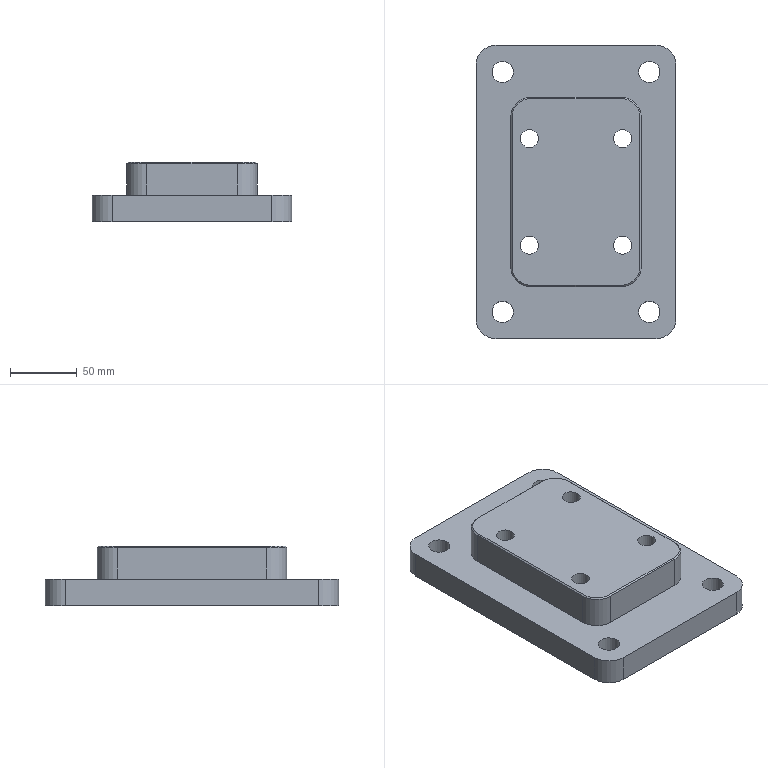Part | 1 solid | 47 faces | box 150 x 220 x 45 mm | volume 944811 mm3 | cylinder 20 | plane 19 | cone 8 | commonest cylinder face diameters 30 x8 13.5 x4 16 x4 20 x4
STEP:
#1=CARTESIAN_POINT('',(-49.,56.,-25.));
#2=VERTEX_POINT('',#1);
#3=CARTESIAN_POINT('',(-49.,56.,-1.));
#4=VERTEX_POINT('',#3);
#5=CARTESIAN_POINT('',(-49.,56.,-25.));
#6=DIRECTION('',(0.,0.,1.));
#7=VECTOR('',#6,1000.);
#8=LINE('',#5,#7);
#9=EDGE_CURVE('',#2,#4,#8,.T.);
#10=ORIENTED_EDGE('',*,*,#9,.T.);
#11=CARTESIAN_POINT('',(-34.,71.,-1.));
#12=VERTEX_POINT('',#11);
#13=CARTESIAN_POINT('',(-34.,56.,-1.));
#14=DIRECTION('',(0.,0.,1.));
#15=DIRECTION('',(1.,0.,0.));
#16=AXIS2_PLACEMENT_3D('',#13,#14,#15);
#17=CIRCLE('',#16,15.);
#18=EDGE_CURVE('',#4,#12,#17,.F.);
#19=ORIENTED_EDGE('',*,*,#18,.T.);
#20=CARTESIAN_POINT('',(-34.,71.,-25.));
#21=VERTEX_POINT('',#20);
#22=CARTESIAN_POINT('',(-34.,71.,-25.));
#23=DIRECTION('',(0.,0.,1.));
#24=VECTOR('',#23,1000.);
#25=LINE('',#22,#24);
#26=EDGE_CURVE('',#21,#12,#25,.T.);
#27=ORIENTED_EDGE('',*,*,#26,.F.);
#28=CARTESIAN_POINT('',(-34.,56.,-25.));
#29=DIRECTION('',(0.,0.,-1.));
#30=DIRECTION('',(1.,0.,0.));
#31=AXIS2_PLACEMENT_3D('',#28,#29,#30);
#32=CIRCLE('',#31,15.);
#33=EDGE_CURVE('',#2,#21,#32,.T.);
#34=ORIENTED_EDGE('',*,*,#33,.F.);
#35=EDGE_LOOP('',(#10,#19,#27,#34));
#36=FACE_BOUND('',#35,.T.);
#37=CARTESIAN_POINT('',(-34.,56.,-25.));
#38=DIRECTION('',(0.,0.,1.));
#39=DIRECTION('',(1.,0.,0.));
#40=AXIS2_PLACEMENT_3D('',#37,#38,#39);
#41=CYLINDRICAL_SURFACE('',#40,15.);
#42=ADVANCED_FACE('',(#36),#41,.T.);
#43=ORIENTED_EDGE('',*,*,#26,.T.);
#44=CARTESIAN_POINT('',(34.,71.,-1.));
#45=VERTEX_POINT('',#44);
#46=CARTESIAN_POINT('',(34.,71.,-1.));
#47=DIRECTION('',(1.,0.,0.));
#48=VECTOR('',#47,1000.);
#49=LINE('',#46,#48);
#50=EDGE_CURVE('',#12,#45,#49,.T.);
#51=ORIENTED_EDGE('',*,*,#50,.T.);
#52=CARTESIAN_POINT('',(34.,71.,-25.));
#53=VERTEX_POINT('',#52);
#54=CARTESIAN_POINT('',(34.,71.,-25.));
#55=DIRECTION('',(0.,0.,1.));
#56=VECTOR('',#55,1000.);
#57=LINE('',#54,#56);
#58=EDGE_CURVE('',#53,#45,#57,.T.);
#59=ORIENTED_EDGE('',*,*,#58,.F.);
#60=CARTESIAN_POINT('',(34.,71.,-25.));
#61=DIRECTION('',(1.,0.,0.));
#62=VECTOR('',#61,1000.);
#63=LINE('',#60,#62);
#64=EDGE_CURVE('',#21,#53,#63,.T.);
#65=ORIENTED_EDGE('',*,*,#64,.F.);
#66=EDGE_LOOP('',(#43,#51,#59,#65));
#67=FACE_BOUND('',#66,.T.);
#68=CARTESIAN_POINT('',(34.,71.,-25.));
#69=DIRECTION('',(0.,-1.,0.));
#70=DIRECTION('',(0.,0.,1.));
#71=AXIS2_PLACEMENT_3D('',#68,#69,#70);
#72=PLANE('',#71);
#73=ADVANCED_FACE('',(#67),#72,.F.);
#74=ORIENTED_EDGE('',*,*,#58,.T.);
#75=CARTESIAN_POINT('',(49.,56.,-1.));
#76=VERTEX_POINT('',#75);
#77=CARTESIAN_POINT('',(34.,56.,-1.));
#78=DIRECTION('',(0.,0.,1.));
#79=DIRECTION('',(1.,0.,0.));
#80=AXIS2_PLACEMENT_3D('',#77,#78,#79);
#81=CIRCLE('',#80,15.);
#82=EDGE_CURVE('',#45,#76,#81,.F.);
#83=ORIENTED_EDGE('',*,*,#82,.T.);
#84=CARTESIAN_POINT('',(49.,56.,-25.));
#85=VERTEX_POINT('',#84);
#86=CARTESIAN_POINT('',(49.,56.,-25.));
#87=DIRECTION('',(0.,0.,1.));
#88=VECTOR('',#87,1000.);
#89=LINE('',#86,#88);
#90=EDGE_CURVE('',#85,#76,#89,.T.);
#91=ORIENTED_EDGE('',*,*,#90,.F.);
#92=CARTESIAN_POINT('',(34.,56.,-25.));
#93=DIRECTION('',(0.,0.,-1.));
#94=DIRECTION('',(-1.,0.,0.));
#95=AXIS2_PLACEMENT_3D('',#92,#93,#94);
#96=CIRCLE('',#95,15.);
#97=EDGE_CURVE('',#53,#85,#96,.T.);
#98=ORIENTED_EDGE('',*,*,#97,.F.);
#99=EDGE_LOOP('',(#74,#83,#91,#98));
#100=FACE_BOUND('',#99,.T.);
#101=CARTESIAN_POINT('',(34.,56.,-25.));
#102=DIRECTION('',(0.,0.,1.));
#103=DIRECTION('',(1.,0.,0.));
#104=AXIS2_PLACEMENT_3D('',#101,#102,#103);
#105=CYLINDRICAL_SURFACE('',#104,15.);
#106=ADVANCED_FACE('',(#100),#105,.T.);
#107=ORIENTED_EDGE('',*,*,#90,.T.);
#108=CARTESIAN_POINT('',(49.,-56.,-1.));
#109=VERTEX_POINT('',#108);
#110=CARTESIAN_POINT('',(49.,-56.,-1.));
#111=DIRECTION('',(0.,-1.,0.));
#112=VECTOR('',#111,1000.);
#113=LINE('',#110,#112);
#114=EDGE_CURVE('',#76,#109,#113,.T.);
#115=ORIENTED_EDGE('',*,*,#114,.T.);
#116=CARTESIAN_POINT('',(49.,-56.,-25.));
#117=VERTEX_POINT('',#116);
#118=CARTESIAN_POINT('',(49.,-56.,-25.));
#119=DIRECTION('',(0.,0.,1.));
#120=VECTOR('',#119,1000.);
#121=LINE('',#118,#120);
#122=EDGE_CURVE('',#117,#109,#121,.T.);
#123=ORIENTED_EDGE('',*,*,#122,.F.);
#124=CARTESIAN_POINT('',(49.,56.,-25.));
#125=DIRECTION('',(0.,-1.,0.));
#126=VECTOR('',#125,1000.);
#127=LINE('',#124,#126);
#128=EDGE_CURVE('',#85,#117,#127,.T.);
#129=ORIENTED_EDGE('',*,*,#128,.F.);
#130=EDGE_LOOP('',(#107,#115,#123,#129));
#131=FACE_BOUND('',#130,.T.);
#132=CARTESIAN_POINT('',(49.,56.,-25.));
#133=DIRECTION('',(-1.,0.,0.));
#134=DIRECTION('',(0.,1.,0.));
#135=AXIS2_PLACEMENT_3D('',#132,#133,#134);
#136=PLANE('',#135);
#137=ADVANCED_FACE('',(#131),#136,.F.);
#138=ORIENTED_EDGE('',*,*,#122,.T.);
#139=CARTESIAN_POINT('',(34.,-71.,-1.));
#140=VERTEX_POINT('',#139);
#141=CARTESIAN_POINT('',(34.,-56.,-1.));
#142=DIRECTION('',(0.,0.,1.));
#143=DIRECTION('',(1.,0.,0.));
#144=AXIS2_PLACEMENT_3D('',#141,#142,#143);
#145=CIRCLE('',#144,15.);
#146=EDGE_CURVE('',#109,#140,#145,.F.);
#147=ORIENTED_EDGE('',*,*,#146,.T.);
#148=CARTESIAN_POINT('',(34.,-71.,-25.));
#149=VERTEX_POINT('',#148);
#150=CARTESIAN_POINT('',(34.,-71.,-25.));
#151=DIRECTION('',(0.,0.,1.));
#152=VECTOR('',#151,1000.);
#153=LINE('',#150,#152);
#154=EDGE_CURVE('',#149,#140,#153,.T.);
#155=ORIENTED_EDGE('',*,*,#154,.F.);
#156=CARTESIAN_POINT('',(34.,-56.,-25.));
#157=DIRECTION('',(0.,0.,-1.));
#158=DIRECTION('',(-1.,0.,0.));
#159=AXIS2_PLACEMENT_3D('',#156,#157,#158);
#160=CIRCLE('',#159,15.);
#161=EDGE_CURVE('',#117,#149,#160,.T.);
#162=ORIENTED_EDGE('',*,*,#161,.F.);
#163=EDGE_LOOP('',(#138,#147,#155,#162));
#164=FACE_BOUND('',#163,.T.);
#165=CARTESIAN_POINT('',(34.,-56.,-25.));
#166=DIRECTION('',(0.,0.,1.));
#167=DIRECTION('',(1.,0.,0.));
#168=AXIS2_PLACEMENT_3D('',#165,#166,#167);
#169=CYLINDRICAL_SURFACE('',#168,15.);
#170=ADVANCED_FACE('',(#164),#169,.T.);
#171=ORIENTED_EDGE('',*,*,#154,.T.);
#172=CARTESIAN_POINT('',(-34.,-71.,-1.));
#173=VERTEX_POINT('',#172);
#174=CARTESIAN_POINT('',(-34.,-71.,-1.));
#175=DIRECTION('',(-1.,0.,0.));
#176=VECTOR('',#175,1000.);
#177=LINE('',#174,#176);
#178=EDGE_CURVE('',#140,#173,#177,.T.);
#179=ORIENTED_EDGE('',*,*,#178,.T.);
#180=CARTESIAN_POINT('',(-34.,-71.,-25.));
#181=VERTEX_POINT('',#180);
#182=CARTESIAN_POINT('',(-34.,-71.,-25.));
#183=DIRECTION('',(0.,0.,1.));
#184=VECTOR('',#183,1000.);
#185=LINE('',#182,#184);
#186=EDGE_CURVE('',#181,#173,#185,.T.);
#187=ORIENTED_EDGE('',*,*,#186,.F.);
#188=CARTESIAN_POINT('',(34.,-71.,-25.));
#189=DIRECTION('',(-1.,0.,0.));
#190=VECTOR('',#189,1000.);
#191=LINE('',#188,#190);
#192=EDGE_CURVE('',#149,#181,#191,.T.);
#193=ORIENTED_EDGE('',*,*,#192,.F.);
#194=EDGE_LOOP('',(#171,#179,#187,#193));
#195=FACE_BOUND('',#194,.T.);
#196=CARTESIAN_POINT('',(34.,-71.,-25.));
#197=DIRECTION('',(0.,1.,0.));
#198=DIRECTION('',(0.,0.,-1.));
#199=AXIS2_PLACEMENT_3D('',#196,#197,#198);
#200=PLANE('',#199);
#201=ADVANCED_FACE('',(#195),#200,.F.);
#202=ORIENTED_EDGE('',*,*,#186,.T.);
#203=CARTESIAN_POINT('',(-49.,-56.,-1.));
#204=VERTEX_POINT('',#203);
#205=CARTESIAN_POINT('',(-34.,-56.,-1.));
#206=DIRECTION('',(0.,0.,1.));
#207=DIRECTION('',(1.,0.,0.));
#208=AXIS2_PLACEMENT_3D('',#205,#206,#207);
#209=CIRCLE('',#208,15.);
#210=EDGE_CURVE('',#173,#204,#209,.F.);
#211=ORIENTED_EDGE('',*,*,#210,.T.);
#212=CARTESIAN_POINT('',(-49.,-56.,-25.));
#213=VERTEX_POINT('',#212);
#214=CARTESIAN_POINT('',(-49.,-56.,-25.));
#215=DIRECTION('',(0.,0.,1.));
#216=VECTOR('',#215,1000.);
#217=LINE('',#214,#216);
#218=EDGE_CURVE('',#213,#204,#217,.T.);
#219=ORIENTED_EDGE('',*,*,#218,.F.);
#220=CARTESIAN_POINT('',(-34.,-56.,-25.));
#221=DIRECTION('',(0.,0.,-1.));
#222=DIRECTION('',(-1.,0.,0.));
#223=AXIS2_PLACEMENT_3D('',#220,#221,#222);
#224=CIRCLE('',#223,15.);
#225=EDGE_CURVE('',#181,#213,#224,.T.);
#226=ORIENTED_EDGE('',*,*,#225,.F.);
#227=EDGE_LOOP('',(#202,#211,#219,#226));
#228=FACE_BOUND('',#227,.T.);
#229=CARTESIAN_POINT('',(-34.,-56.,-25.));
#230=DIRECTION('',(0.,0.,1.));
#231=DIRECTION('',(1.,0.,0.));
#232=AXIS2_PLACEMENT_3D('',#229,#230,#231);
#233=CYLINDRICAL_SURFACE('',#232,15.);
#234=ADVANCED_FACE('',(#228),#233,.T.);
#235=ORIENTED_EDGE('',*,*,#218,.T.);
#236=CARTESIAN_POINT('',(-49.,56.,-1.));
#237=DIRECTION('',(0.,1.,0.));
#238=VECTOR('',#237,1000.);
#239=LINE('',#236,#238);
#240=EDGE_CURVE('',#204,#4,#239,.T.);
#241=ORIENTED_EDGE('',*,*,#240,.T.);
#242=ORIENTED_EDGE('',*,*,#9,.F.);
#243=CARTESIAN_POINT('',(-49.,56.,-25.));
#244=DIRECTION('',(0.,1.,0.));
#245=VECTOR('',#244,1000.);
#246=LINE('',#243,#245);
#247=EDGE_CURVE('',#213,#2,#246,.T.);
#248=ORIENTED_EDGE('',*,*,#247,.F.);
#249=EDGE_LOOP('',(#235,#241,#242,#248));
#250=FACE_BOUND('',#249,.T.);
#251=CARTESIAN_POINT('',(-49.,56.,-25.));
#252=DIRECTION('',(1.,0.,0.));
#253=DIRECTION('',(0.,-1.,0.));
#254=AXIS2_PLACEMENT_3D('',#251,#252,#253);
#255=PLANE('',#254);
#256=ADVANCED_FACE('',(#250),#255,.F.);
#257=CARTESIAN_POINT('',(28.25,40.,0.));
#258=VERTEX_POINT('',#257);
#259=CARTESIAN_POINT('',(35.,40.,0.));
#260=DIRECTION('',(0.,0.,-1.));
#261=DIRECTION('',(-1.,0.,0.));
#262=AXIS2_PLACEMENT_3D('',#259,#260,#261);
#263=CIRCLE('',#262,6.75);
#264=EDGE_CURVE('',#258,#258,#263,.T.);
#265=ORIENTED_EDGE('',*,*,#264,.T.);
#266=EDGE_LOOP('',(#265));
#267=FACE_BOUND('',#266,.T.);
#268=CARTESIAN_POINT('',(-41.75,40.,0.));
#269=VERTEX_POINT('',#268);
#270=CARTESIAN_POINT('',(-35.,40.,0.));
#271=DIRECTION('',(0.,0.,-1.));
#272=DIRECTION('',(-1.,0.,0.));
#273=AXIS2_PLACEMENT_3D('',#270,#271,#272);
#274=CIRCLE('',#273,6.75);
#275=EDGE_CURVE('',#269,#269,#274,.T.);
#276=ORIENTED_EDGE('',*,*,#275,.T.);
#277=EDGE_LOOP('',(#276));
#278=FACE_BOUND('',#277,.T.);
#279=CARTESIAN_POINT('',(28.25,-40.,0.));
#280=VERTEX_POINT('',#279);
#281=CARTESIAN_POINT('',(35.,-40.,0.));
#282=DIRECTION('',(0.,0.,-1.));
#283=DIRECTION('',(-1.,0.,0.));
#284=AXIS2_PLACEMENT_3D('',#281,#282,#283);
#285=CIRCLE('',#284,6.75);
#286=EDGE_CURVE('',#280,#280,#285,.T.);
#287=ORIENTED_EDGE('',*,*,#286,.T.);
#288=EDGE_LOOP('',(#287));
#289=FACE_BOUND('',#288,.T.);
#290=CARTESIAN_POINT('',(-41.75,-40.,0.));
#291=VERTEX_POINT('',#290);
#292=CARTESIAN_POINT('',(-35.,-40.,0.));
#293=DIRECTION('',(0.,0.,-1.));
#294=DIRECTION('',(-1.,0.,0.));
#295=AXIS2_PLACEMENT_3D('',#292,#293,#294);
#296=CIRCLE('',#295,6.75);
#297=EDGE_CURVE('',#291,#291,#296,.T.);
#298=ORIENTED_EDGE('',*,*,#297,.T.);
#299=EDGE_LOOP('',(#298));
#300=FACE_BOUND('',#299,.T.);
#301=CARTESIAN_POINT('',(-34.,70.,0.));
#302=VERTEX_POINT('',#301);
#303=CARTESIAN_POINT('',(-48.,56.,0.));
#304=VERTEX_POINT('',#303);
#305=CARTESIAN_POINT('',(-34.,56.,0.));
#306=DIRECTION('',(0.,0.,1.));
#307=DIRECTION('',(1.,0.,0.));
#308=AXIS2_PLACEMENT_3D('',#305,#306,#307);
#309=CIRCLE('',#308,14.);
#310=EDGE_CURVE('',#302,#304,#309,.T.);
#311=ORIENTED_EDGE('',*,*,#310,.T.);
#312=CARTESIAN_POINT('',(-48.,-56.,0.));
#313=VERTEX_POINT('',#312);
#314=CARTESIAN_POINT('',(-48.,-56.,0.));
#315=DIRECTION('',(0.,-1.,0.));
#316=VECTOR('',#315,1000.);
#317=LINE('',#314,#316);
#318=EDGE_CURVE('',#304,#313,#317,.T.);
#319=ORIENTED_EDGE('',*,*,#318,.T.);
#320=CARTESIAN_POINT('',(-34.,-70.,0.));
#321=VERTEX_POINT('',#320);
#322=CARTESIAN_POINT('',(-34.,-56.,0.));
#323=DIRECTION('',(0.,0.,1.));
#324=DIRECTION('',(1.,0.,0.));
#325=AXIS2_PLACEMENT_3D('',#322,#323,#324);
#326=CIRCLE('',#325,14.);
#327=EDGE_CURVE('',#313,#321,#326,.T.);
#328=ORIENTED_EDGE('',*,*,#327,.T.);
#329=CARTESIAN_POINT('',(34.,-70.,0.));
#330=VERTEX_POINT('',#329);
#331=CARTESIAN_POINT('',(34.,-70.,0.));
#332=DIRECTION('',(1.,0.,0.));
#333=VECTOR('',#332,1000.);
#334=LINE('',#331,#333);
#335=EDGE_CURVE('',#321,#330,#334,.T.);
#336=ORIENTED_EDGE('',*,*,#335,.T.);
#337=CARTESIAN_POINT('',(48.,-56.,0.));
#338=VERTEX_POINT('',#337);
#339=CARTESIAN_POINT('',(34.,-56.,0.));
#340=DIRECTION('',(0.,0.,1.));
#341=DIRECTION('',(1.,0.,0.));
#342=AXIS2_PLACEMENT_3D('',#339,#340,#341);
#343=CIRCLE('',#342,14.);
#344=EDGE_CURVE('',#330,#338,#343,.T.);
#345=ORIENTED_EDGE('',*,*,#344,.T.);
#346=CARTESIAN_POINT('',(48.,56.,0.));
#347=VERTEX_POINT('',#346);
#348=CARTESIAN_POINT('',(48.,56.,0.));
#349=DIRECTION('',(0.,1.,0.));
#350=VECTOR('',#349,1000.);
#351=LINE('',#348,#350);
#352=EDGE_CURVE('',#338,#347,#351,.T.);
#353=ORIENTED_EDGE('',*,*,#352,.T.);
#354=CARTESIAN_POINT('',(34.,70.,0.));
#355=VERTEX_POINT('',#354);
#356=CARTESIAN_POINT('',(34.,56.,0.));
#357=DIRECTION('',(0.,0.,1.));
#358=DIRECTION('',(1.,0.,0.));
#359=AXIS2_PLACEMENT_3D('',#356,#357,#358);
#360=CIRCLE('',#359,14.);
#361=EDGE_CURVE('',#347,#355,#360,.T.);
#362=ORIENTED_EDGE('',*,*,#361,.T.);
#363=CARTESIAN_POINT('',(-34.,70.,0.));
#364=DIRECTION('',(-1.,0.,0.));
#365=VECTOR('',#364,1000.);
#366=LINE('',#363,#365);
#367=EDGE_CURVE('',#355,#302,#366,.T.);
#368=ORIENTED_EDGE('',*,*,#367,.T.);
#369=EDGE_LOOP('',(#311,#319,#328,#336,#345,#353,#362,#368));
#370=FACE_BOUND('',#369,.T.);
#371=CARTESIAN_POINT('',(-34.,56.,0.));
#372=DIRECTION('',(0.,0.,1.));
#373=DIRECTION('',(1.,0.,0.));
#374=AXIS2_PLACEMENT_3D('',#371,#372,#373);
#375=PLANE('',#374);
#376=ADVANCED_FACE('',(#267,#278,#289,#300,#370),#375,.T.);
#377=CARTESIAN_POINT('',(75.,95.,-25.));
#378=VERTEX_POINT('',#377);
#379=CARTESIAN_POINT('',(75.,-95.,-25.));
#380=VERTEX_POINT('',#379);
#381=CARTESIAN_POINT('',(75.,110.,-25.));
#382=DIRECTION('',(0.,-1.,0.));
#383=VECTOR('',#382,1000.);
#384=LINE('',#381,#383);
#385=EDGE_CURVE('',#378,#380,#384,.T.);
#386=ORIENTED_EDGE('',*,*,#385,.T.);
#387=CARTESIAN_POINT('',(75.,-95.,-45.));
#388=VERTEX_POINT('',#387);
#389=CARTESIAN_POINT('',(75.,-95.,-45.));
#390=DIRECTION('',(0.,0.,1.));
#391=VECTOR('',#390,1000.);
#392=LINE('',#389,#391);
#393=EDGE_CURVE('',#380,#388,#392,.F.);
#394=ORIENTED_EDGE('',*,*,#393,.T.);
#395=CARTESIAN_POINT('',(75.,95.,-45.));
#396=VERTEX_POINT('',#395);
#397=CARTESIAN_POINT('',(75.,110.,-45.));
#398=DIRECTION('',(0.,-1.,0.));
#399=VECTOR('',#398,1000.);
#400=LINE('',#397,#399);
#401=EDGE_CURVE('',#396,#388,#400,.T.);
#402=ORIENTED_EDGE('',*,*,#401,.F.);
#403=CARTESIAN_POINT('',(75.,95.,-45.));
#404=DIRECTION('',(0.,0.,1.));
#405=VECTOR('',#404,1000.);
#406=LINE('',#403,#405);
#407=EDGE_CURVE('',#396,#378,#406,.T.);
#408=ORIENTED_EDGE('',*,*,#407,.T.);
#409=EDGE_LOOP('',(#386,#394,#402,#408));
#410=FACE_BOUND('',#409,.T.);
#411=CARTESIAN_POINT('',(75.,110.,-45.));
#412=DIRECTION('',(-1.,0.,0.));
#413=DIRECTION('',(0.,1.,0.));
#414=AXIS2_PLACEMENT_3D('',#411,#412,#413);
#415=PLANE('',#414);
#416=ADVANCED_FACE('',(#410),#415,.F.);
#417=CARTESIAN_POINT('',(60.,-110.,-25.));
#418=VERTEX_POINT('',#417);
#419=CARTESIAN_POINT('',(-60.,-110.,-25.));
#420=VERTEX_POINT('',#419);
#421=CARTESIAN_POINT('',(-75.,-110.,-25.));
#422=DIRECTION('',(-1.,0.,0.));
#423=VECTOR('',#422,1000.);
#424=LINE('',#421,#423);
#425=EDGE_CURVE('',#418,#420,#424,.T.);
#426=ORIENTED_EDGE('',*,*,#425,.T.);
#427=CARTESIAN_POINT('',(-60.,-110.,-45.));
#428=VERTEX_POINT('',#427);
#429=CARTESIAN_POINT('',(-60.,-110.,-45.));
#430=DIRECTION('',(0.,0.,1.));
#431=VECTOR('',#430,1000.);
#432=LINE('',#429,#431);
#433=EDGE_CURVE('',#420,#428,#432,.F.);
#434=ORIENTED_EDGE('',*,*,#433,.T.);
#435=CARTESIAN_POINT('',(60.,-110.,-45.));
#436=VERTEX_POINT('',#435);
#437=CARTESIAN_POINT('',(-75.,-110.,-45.));
#438=DIRECTION('',(-1.,0.,0.));
#439=VECTOR('',#438,1000.);
#440=LINE('',#437,#439);
#441=EDGE_CURVE('',#436,#428,#440,.T.);
#442=ORIENTED_EDGE('',*,*,#441,.F.);
#443=CARTESIAN_POINT('',(60.,-110.,-45.));
#444=DIRECTION('',(0.,0.,1.));
#445=VECTOR('',#444,1000.);
#446=LINE('',#443,#445);
#447=EDGE_CURVE('',#436,#418,#446,.T.);
#448=ORIENTED_EDGE('',*,*,#447,.T.);
#449=EDGE_LOOP('',(#426,#434,#442,#448));
#450=FACE_BOUND('',#449,.T.);
#451=CARTESIAN_POINT('',(-75.,-110.,-45.));
#452=DIRECTION('',(0.,1.,0.));
#453=DIRECTION('',(1.,0.,0.));
#454=AXIS2_PLACEMENT_3D('',#451,#452,#453);
#455=PLANE('',#454);
#456=ADVANCED_FACE('',(#450),#455,.F.);
#457=CARTESIAN_POINT('',(-75.,-95.,-45.));
#458=VERTEX_POINT('',#457);
#459=CARTESIAN_POINT('',(-75.,95.,-45.));
#460=VERTEX_POINT('',#459);
#461=CARTESIAN_POINT('',(-75.,110.,-45.));
#462=DIRECTION('',(0.,1.,0.));
#463=VECTOR('',#462,1000.);
#464=LINE('',#461,#463);
#465=EDGE_CURVE('',#458,#460,#464,.T.);
#466=ORIENTED_EDGE('',*,*,#465,.F.);
#467=CARTESIAN_POINT('',(-75.,-95.,-25.));
#468=VERTEX_POINT('',#467);
#469=CARTESIAN_POINT('',(-75.,-95.,-45.));
#470=DIRECTION('',(0.,0.,1.));
#471=VECTOR('',#470,1000.);
#472=LINE('',#469,#471);
#473=EDGE_CURVE('',#458,#468,#472,.T.);
#474=ORIENTED_EDGE('',*,*,#473,.T.);
#475=CARTESIAN_POINT('',(-75.,95.,-25.));
#476=VERTEX_POINT('',#475);
#477=CARTESIAN_POINT('',(-75.,110.,-25.));
#478=DIRECTION('',(0.,1.,0.));
#479=VECTOR('',#478,1000.);
#480=LINE('',#477,#479);
#481=EDGE_CURVE('',#468,#476,#480,.T.);
#482=ORIENTED_EDGE('',*,*,#481,.T.);
#483=CARTESIAN_POINT('',(-75.,95.,-45.));
#484=DIRECTION('',(0.,0.,1.));
#485=VECTOR('',#484,1000.);
#486=LINE('',#483,#485);
#487=EDGE_CURVE('',#476,#460,#486,.F.);
#488=ORIENTED_EDGE('',*,*,#487,.T.);
#489=EDGE_LOOP('',(#466,#474,#482,#488));
#490=FACE_BOUND('',#489,.T.);
#491=CARTESIAN_POINT('',(-75.,110.,-45.));
#492=DIRECTION('',(1.,0.,0.));
#493=DIRECTION('',(0.,-1.,0.));
#494=AXIS2_PLACEMENT_3D('',#491,#492,#493);
#495=PLANE('',#494);
#496=ADVANCED_FACE('',(#490),#495,.F.);
#497=CARTESIAN_POINT('',(-60.,110.,-45.));
#498=VERTEX_POINT('',#497);
#499=CARTESIAN_POINT('',(60.,110.,-45.));
#500=VERTEX_POINT('',#499);
#501=CARTESIAN_POINT('',(-75.,110.,-45.));
#502=DIRECTION('',(1.,0.,0.));
#503=VECTOR('',#502,1000.);
#504=LINE('',#501,#503);
#505=EDGE_CURVE('',#498,#500,#504,.T.);
#506=ORIENTED_EDGE('',*,*,#505,.F.);
#507=CARTESIAN_POINT('',(-60.,110.,-25.));
#508=VERTEX_POINT('',#507);
#509=CARTESIAN_POINT('',(-60.,110.,-45.));
#510=DIRECTION('',(0.,0.,1.));
#511=VECTOR('',#510,1000.);
#512=LINE('',#509,#511);
#513=EDGE_CURVE('',#498,#508,#512,.T.);
#514=ORIENTED_EDGE('',*,*,#513,.T.);
#515=CARTESIAN_POINT('',(60.,110.,-25.));
#516=VERTEX_POINT('',#515);
#517=CARTESIAN_POINT('',(-75.,110.,-25.));
#518=DIRECTION('',(1.,0.,0.));
#519=VECTOR('',#518,1000.);
#520=LINE('',#517,#519);
#521=EDGE_CURVE('',#508,#516,#520,.T.);
#522=ORIENTED_EDGE('',*,*,#521,.T.);
#523=CARTESIAN_POINT('',(60.,110.,-45.));
#524=DIRECTION('',(0.,0.,1.));
#525=VECTOR('',#524,1000.);
#526=LINE('',#523,#525);
#527=EDGE_CURVE('',#516,#500,#526,.F.);
#528=ORIENTED_EDGE('',*,*,#527,.T.);
#529=EDGE_LOOP('',(#506,#514,#522,#528));
#530=FACE_BOUND('',#529,.T.);
#531=CARTESIAN_POINT('',(-75.,110.,-45.));
#532=DIRECTION('',(0.,-1.,0.));
#533=DIRECTION('',(-1.,0.,0.));
#534=AXIS2_PLACEMENT_3D('',#531,#532,#533);
#535=PLANE('',#534);
#536=ADVANCED_FACE('',(#530),#535,.F.);
#537=CARTESIAN_POINT('',(24.75,40.,-45.));
#538=VERTEX_POINT('',#537);
#539=CARTESIAN_POINT('',(35.,40.,-45.));
#540=DIRECTION('',(0.,0.,-1.));
#541=DIRECTION('',(-1.,0.,0.));
#542=AXIS2_PLACEMENT_3D('',#539,#540,#541);
#543=CIRCLE('',#542,10.25);
#544=EDGE_CURVE('',#538,#538,#543,.T.);
#545=ORIENTED_EDGE('',*,*,#544,.F.);
#546=EDGE_LOOP('',(#545));
#547=FACE_BOUND('',#546,.T.);
#548=CARTESIAN_POINT('',(-45.25,40.,-45.));
#549=VERTEX_POINT('',#548);
#550=CARTESIAN_POINT('',(-35.,40.,-45.));
#551=DIRECTION('',(0.,0.,-1.));
#552=DIRECTION('',(-1.,0.,0.));
#553=AXIS2_PLACEMENT_3D('',#550,#551,#552);
#554=CIRCLE('',#553,10.25);
#555=EDGE_CURVE('',#549,#549,#554,.T.);
#556=ORIENTED_EDGE('',*,*,#555,.F.);
#557=EDGE_LOOP('',(#556));
#558=FACE_BOUND('',#557,.T.);
#559=CARTESIAN_POINT('',(24.75,-40.,-45.));
#560=VERTEX_POINT('',#559);
#561=CARTESIAN_POINT('',(35.,-40.,-45.));
#562=DIRECTION('',(0.,0.,-1.));
#563=DIRECTION('',(-1.,0.,0.));
#564=AXIS2_PLACEMENT_3D('',#561,#562,#563);
#565=CIRCLE('',#564,10.25);
#566=EDGE_CURVE('',#560,#560,#565,.T.);
#567=ORIENTED_EDGE('',*,*,#566,.F.);
#568=EDGE_LOOP('',(#567));
#569=FACE_BOUND('',#568,.T.);
#570=CARTESIAN_POINT('',(-45.25,-40.,-45.));
#571=VERTEX_POINT('',#570);
#572=CARTESIAN_POINT('',(-35.,-40.,-45.));
#573=DIRECTION('',(0.,0.,-1.));
#574=DIRECTION('',(-1.,0.,0.));
#575=AXIS2_PLACEMENT_3D('',#572,#573,#574);
#576=CIRCLE('',#575,10.25);
#577=EDGE_CURVE('',#571,#571,#576,.T.);
#578=ORIENTED_EDGE('',*,*,#577,.F.);
#579=EDGE_LOOP('',(#578));
#580=FACE_BOUND('',#579,.T.);
#581=CARTESIAN_POINT('',(47.,90.,-45.));
#582=VERTEX_POINT('',#581);
#583=CARTESIAN_POINT('',(55.,90.,-45.));
#584=DIRECTION('',(0.,0.,1.));
#585=DIRECTION('',(-1.,0.,0.));
#586=AXIS2_PLACEMENT_3D('',#583,#584,#585);
#587=CIRCLE('',#586,8.);
#588=EDGE_CURVE('',#582,#582,#587,.T.);
#589=ORIENTED_EDGE('',*,*,#588,.T.);
#590=EDGE_LOOP('',(#589));
#591=FACE_BOUND('',#590,.T.);
#592=CARTESIAN_POINT('',(-47.,90.,-45.));
#593=VERTEX_POINT('',#592);
#594=CARTESIAN_POINT('',(-55.,90.,-45.));
#595=DIRECTION('',(0.,0.,1.));
#596=DIRECTION('',(1.,0.,0.));
#597=AXIS2_PLACEMENT_3D('',#594,#595,#596);
#598=CIRCLE('',#597,8.);
#599=EDGE_CURVE('',#593,#593,#598,.T.);
#600=ORIENTED_EDGE('',*,*,#599,.T.);
#601=EDGE_LOOP('',(#600));
#602=FACE_BOUND('',#601,.T.);
#603=CARTESIAN_POINT('',(-63.,-90.,-45.));
#604=VERTEX_POINT('',#603);
#605=CARTESIAN_POINT('',(-55.,-90.,-45.));
#606=DIRECTION('',(0.,0.,1.));
#607=DIRECTION('',(-1.,0.,0.));
#608=AXIS2_PLACEMENT_3D('',#605,#606,#607);
#609=CIRCLE('',#608,8.);
#610=EDGE_CURVE('',#604,#604,#609,.T.);
#611=ORIENTED_EDGE('',*,*,#610,.T.);
#612=EDGE_LOOP('',(#611));
#613=FACE_BOUND('',#612,.T.);
#614=CARTESIAN_POINT('',(63.,-90.,-45.));
#615=VERTEX_POINT('',#614);
#616=CARTESIAN_POINT('',(55.,-90.,-45.));
#617=DIRECTION('',(0.,0.,1.));
#618=DIRECTION('',(1.,0.,0.));
#619=AXIS2_PLACEMENT_3D('',#616,#617,#618);
#620=CIRCLE('',#619,8.);
#621=EDGE_CURVE('',#615,#615,#620,.T.);
#622=ORIENTED_EDGE('',*,*,#621,.T.);
#623=EDGE_LOOP('',(#622));
#624=FACE_BOUND('',#623,.T.);
#625=ORIENTED_EDGE('',*,*,#441,.T.);
#626=CARTESIAN_POINT('',(-60.,-95.,-45.));
#627=DIRECTION('',(0.,0.,1.));
#628=DIRECTION('',(1.,0.,0.));
#629=AXIS2_PLACEMENT_3D('',#626,#627,#628);
#630=CIRCLE('',#629,15.);
#631=EDGE_CURVE('',#428,#458,#630,.F.);
#632=ORIENTED_EDGE('',*,*,#631,.T.);
#633=ORIENTED_EDGE('',*,*,#465,.T.);
#634=CARTESIAN_POINT('',(-60.,95.,-45.));
#635=DIRECTION('',(0.,0.,1.));
#636=DIRECTION('',(1.,0.,0.));
#637=AXIS2_PLACEMENT_3D('',#634,#635,#636);
#638=CIRCLE('',#637,15.);
#639=EDGE_CURVE('',#460,#498,#638,.F.);
#640=ORIENTED_EDGE('',*,*,#639,.T.);
#641=ORIENTED_EDGE('',*,*,#505,.T.);
#642=CARTESIAN_POINT('',(60.,95.,-45.));
#643=DIRECTION('',(0.,0.,1.));
#644=DIRECTION('',(1.,0.,0.));
#645=AXIS2_PLACEMENT_3D('',#642,#643,#644);
#646=CIRCLE('',#645,15.);
#647=EDGE_CURVE('',#500,#396,#646,.F.);
#648=ORIENTED_EDGE('',*,*,#647,.T.);
#649=ORIENTED_EDGE('',*,*,#401,.T.);
#650=CARTESIAN_POINT('',(60.,-95.,-45.));
#651=DIRECTION('',(0.,0.,1.));
#652=DIRECTION('',(1.,0.,0.));
#653=AXIS2_PLACEMENT_3D('',#650,#651,#652);
#654=CIRCLE('',#653,15.);
#655=EDGE_CURVE('',#388,#436,#654,.F.);
#656=ORIENTED_EDGE('',*,*,#655,.T.);
#657=EDGE_LOOP('',(#625,#632,#633,#640,#641,#648,#649,#656));
#658=FACE_BOUND('',#657,.T.);
#659=CARTESIAN_POINT('',(0.,0.,-45.));
#660=DIRECTION('',(0.,0.,1.));
#661=DIRECTION('',(1.,0.,0.));
#662=AXIS2_PLACEMENT_3D('',#659,#660,#661);
#663=PLANE('',#662);
#664=ADVANCED_FACE('',(#547,#558,#569,#580,#591,#602,#613,#624,#658),#663,.F.);
#665=CARTESIAN_POINT('',(47.,90.,-25.));
#666=VERTEX_POINT('',#665);
#667=CARTESIAN_POINT('',(55.,90.,-25.));
#668=DIRECTION('',(0.,0.,1.));
#669=DIRECTION('',(-1.,0.,0.));
#670=AXIS2_PLACEMENT_3D('',#667,#668,#669);
#671=CIRCLE('',#670,8.);
#672=EDGE_CURVE('',#666,#666,#671,.T.);
#673=ORIENTED_EDGE('',*,*,#672,.F.);
#674=EDGE_LOOP('',(#673));
#675=FACE_BOUND('',#674,.T.);
#676=CARTESIAN_POINT('',(-47.,90.,-25.));
#677=VERTEX_POINT('',#676);
#678=CARTESIAN_POINT('',(-55.,90.,-25.));
#679=DIRECTION('',(0.,0.,1.));
#680=DIRECTION('',(1.,0.,0.));
#681=AXIS2_PLACEMENT_3D('',#678,#679,#680);
#682=CIRCLE('',#681,8.);
#683=EDGE_CURVE('',#677,#677,#682,.T.);
#684=ORIENTED_EDGE('',*,*,#683,.F.);
#685=EDGE_LOOP('',(#684));
#686=FACE_BOUND('',#685,.T.);
#687=CARTESIAN_POINT('',(-63.,-90.,-25.));
#688=VERTEX_POINT('',#687);
#689=CARTESIAN_POINT('',(-55.,-90.,-25.));
#690=DIRECTION('',(0.,0.,1.));
#691=DIRECTION('',(-1.,0.,0.));
#692=AXIS2_PLACEMENT_3D('',#689,#690,#691);
#693=CIRCLE('',#692,8.);
#694=EDGE_CURVE('',#688,#688,#693,.T.);
#695=ORIENTED_EDGE('',*,*,#694,.F.);
#696=EDGE_LOOP('',(#695));
#697=FACE_BOUND('',#696,.T.);
#698=CARTESIAN_POINT('',(63.,-90.,-25.));
#699=VERTEX_POINT('',#698);
#700=CARTESIAN_POINT('',(55.,-90.,-25.));
#701=DIRECTION('',(0.,0.,1.));
#702=DIRECTION('',(1.,0.,0.));
#703=AXIS2_PLACEMENT_3D('',#700,#701,#702);
#704=CIRCLE('',#703,8.);
#705=EDGE_CURVE('',#699,#699,#704,.T.);
#706=ORIENTED_EDGE('',*,*,#705,.F.);
#707=EDGE_LOOP('',(#706));
#708=FACE_BOUND('',#707,.T.);
#709=ORIENTED_EDGE('',*,*,#247,.T.);
#710=ORIENTED_EDGE('',*,*,#33,.T.);
#711=ORIENTED_EDGE('',*,*,#64,.T.);
#712=ORIENTED_EDGE('',*,*,#97,.T.);
#713=ORIENTED_EDGE('',*,*,#128,.T.);
#714=ORIENTED_EDGE('',*,*,#161,.T.);
#715=ORIENTED_EDGE('',*,*,#192,.T.);
#716=ORIENTED_EDGE('',*,*,#225,.T.);
#717=EDGE_LOOP('',(#709,#710,#711,#712,#713,#714,#715,#716));
#718=FACE_BOUND('',#717,.T.);
#719=ORIENTED_EDGE('',*,*,#481,.F.);
#720=CARTESIAN_POINT('',(-60.,-95.,-25.));
#721=DIRECTION('',(0.,0.,1.));
#722=DIRECTION('',(1.,0.,0.));
#723=AXIS2_PLACEMENT_3D('',#720,#721,#722);
#724=CIRCLE('',#723,15.);
#725=EDGE_CURVE('',#468,#420,#724,.T.);
#726=ORIENTED_EDGE('',*,*,#725,.T.);
#727=ORIENTED_EDGE('',*,*,#425,.F.);
#728=CARTESIAN_POINT('',(60.,-95.,-25.));
#729=DIRECTION('',(0.,0.,1.));
#730=DIRECTION('',(1.,0.,0.));
#731=AXIS2_PLACEMENT_3D('',#728,#729,#730);
#732=CIRCLE('',#731,15.);
#733=EDGE_CURVE('',#418,#380,#732,.T.);
#734=ORIENTED_EDGE('',*,*,#733,.T.);
#735=ORIENTED_EDGE('',*,*,#385,.F.);
#736=CARTESIAN_POINT('',(60.,95.,-25.));
#737=DIRECTION('',(0.,0.,1.));
#738=DIRECTION('',(1.,0.,0.));
#739=AXIS2_PLACEMENT_3D('',#736,#737,#738);
#740=CIRCLE('',#739,15.);
#741=EDGE_CURVE('',#378,#516,#740,.T.);
#742=ORIENTED_EDGE('',*,*,#741,.T.);
#743=ORIENTED_EDGE('',*,*,#521,.F.);
#744=CARTESIAN_POINT('',(-60.,95.,-25.));
#745=DIRECTION('',(0.,0.,1.));
#746=DIRECTION('',(1.,0.,0.));
#747=AXIS2_PLACEMENT_3D('',#744,#745,#746);
#748=CIRCLE('',#747,15.);
#749=EDGE_CURVE('',#508,#476,#748,.T.);
#750=ORIENTED_EDGE('',*,*,#749,.T.);
#751=EDGE_LOOP('',(#719,#726,#727,#734,#735,#742,#743,#750));
#752=FACE_BOUND('',#751,.T.);
#753=CARTESIAN_POINT('',(0.,0.,-25.));
#754=DIRECTION('',(0.,0.,1.));
#755=DIRECTION('',(1.,0.,0.));
#756=AXIS2_PLACEMENT_3D('',#753,#754,#755);
#757=PLANE('',#756);
#758=ADVANCED_FACE('',(#675,#686,#697,#708,#718,#752),#757,.T.);
#759=ORIENTED_EDGE('',*,*,#631,.F.);
#760=ORIENTED_EDGE('',*,*,#433,.F.);
#761=ORIENTED_EDGE('',*,*,#725,.F.);
#762=ORIENTED_EDGE('',*,*,#473,.F.);
#763=EDGE_LOOP('',(#759,#760,#761,#762));
#764=FACE_BOUND('',#763,.T.);
#765=CARTESIAN_POINT('',(-60.,-95.,-45.));
#766=DIRECTION('',(0.,0.,1.));
#767=DIRECTION('',(1.,0.,0.));
#768=AXIS2_PLACEMENT_3D('',#765,#766,#767);
#769=CYLINDRICAL_SURFACE('',#768,15.);
#770=ADVANCED_FACE('',(#764),#769,.T.);
#771=ORIENTED_EDGE('',*,*,#655,.F.);
#772=ORIENTED_EDGE('',*,*,#393,.F.);
#773=ORIENTED_EDGE('',*,*,#733,.F.);
#774=ORIENTED_EDGE('',*,*,#447,.F.);
#775=EDGE_LOOP('',(#771,#772,#773,#774));
#776=FACE_BOUND('',#775,.T.);
#777=CARTESIAN_POINT('',(60.,-95.,-45.));
#778=DIRECTION('',(0.,0.,1.));
#779=DIRECTION('',(1.,0.,0.));
#780=AXIS2_PLACEMENT_3D('',#777,#778,#779);
#781=CYLINDRICAL_SURFACE('',#780,15.);
#782=ADVANCED_FACE('',(#776),#781,.T.);
#783=ORIENTED_EDGE('',*,*,#639,.F.);
#784=ORIENTED_EDGE('',*,*,#487,.F.);
#785=ORIENTED_EDGE('',*,*,#749,.F.);
#786=ORIENTED_EDGE('',*,*,#513,.F.);
#787=EDGE_LOOP('',(#783,#784,#785,#786));
#788=FACE_BOUND('',#787,.T.);
#789=CARTESIAN_POINT('',(-60.,95.,-45.));
#790=DIRECTION('',(0.,0.,1.));
#791=DIRECTION('',(1.,0.,0.));
#792=AXIS2_PLACEMENT_3D('',#789,#790,#791);
#793=CYLINDRICAL_SURFACE('',#792,15.);
#794=ADVANCED_FACE('',(#788),#793,.T.);
#795=ORIENTED_EDGE('',*,*,#647,.F.);
#796=ORIENTED_EDGE('',*,*,#527,.F.);
#797=ORIENTED_EDGE('',*,*,#741,.F.);
#798=ORIENTED_EDGE('',*,*,#407,.F.);
#799=EDGE_LOOP('',(#795,#796,#797,#798));
#800=FACE_BOUND('',#799,.T.);
#801=CARTESIAN_POINT('',(60.,95.,-45.));
#802=DIRECTION('',(0.,0.,1.));
#803=DIRECTION('',(1.,0.,0.));
#804=AXIS2_PLACEMENT_3D('',#801,#802,#803);
#805=CYLINDRICAL_SURFACE('',#804,15.);
#806=ADVANCED_FACE('',(#800),#805,.T.);
#807=ORIENTED_EDGE('',*,*,#621,.F.);
#808=EDGE_LOOP('',(#807));
#809=FACE_BOUND('',#808,.T.);
#810=ORIENTED_EDGE('',*,*,#705,.T.);
#811=EDGE_LOOP('',(#810));
#812=FACE_BOUND('',#811,.T.);
#813=CARTESIAN_POINT('',(55.,-90.,-45.));
#814=DIRECTION('',(0.,0.,1.));
#815=DIRECTION('',(1.,0.,0.));
#816=AXIS2_PLACEMENT_3D('',#813,#814,#815);
#817=CYLINDRICAL_SURFACE('',#816,8.);
#818=ADVANCED_FACE('',(#809,#812),#817,.F.);
#819=ORIENTED_EDGE('',*,*,#610,.F.);
#820=EDGE_LOOP('',(#819));
#821=FACE_BOUND('',#820,.T.);
#822=ORIENTED_EDGE('',*,*,#694,.T.);
#823=EDGE_LOOP('',(#822));
#824=FACE_BOUND('',#823,.T.);
#825=CARTESIAN_POINT('',(-55.,-90.,-45.));
#826=DIRECTION('',(0.,0.,1.));
#827=DIRECTION('',(1.,0.,0.));
#828=AXIS2_PLACEMENT_3D('',#825,#826,#827);
#829=CYLINDRICAL_SURFACE('',#828,8.);
#830=ADVANCED_FACE('',(#821,#824),#829,.F.);
#831=ORIENTED_EDGE('',*,*,#599,.F.);
#832=EDGE_LOOP('',(#831));
#833=FACE_BOUND('',#832,.T.);
#834=ORIENTED_EDGE('',*,*,#683,.T.);
#835=EDGE_LOOP('',(#834));
#836=FACE_BOUND('',#835,.T.);
#837=CARTESIAN_POINT('',(-55.,90.,-45.));
#838=DIRECTION('',(0.,0.,1.));
#839=DIRECTION('',(1.,0.,0.));
#840=AXIS2_PLACEMENT_3D('',#837,#838,#839);
#841=CYLINDRICAL_SURFACE('',#840,8.);
#842=ADVANCED_FACE('',(#833,#836),#841,.F.);
#843=ORIENTED_EDGE('',*,*,#588,.F.);
#844=EDGE_LOOP('',(#843));
#845=FACE_BOUND('',#844,.T.);
#846=ORIENTED_EDGE('',*,*,#672,.T.);
#847=EDGE_LOOP('',(#846));
#848=FACE_BOUND('',#847,.T.);
#849=CARTESIAN_POINT('',(55.,90.,-45.));
#850=DIRECTION('',(0.,0.,1.));
#851=DIRECTION('',(1.,0.,0.));
#852=AXIS2_PLACEMENT_3D('',#849,#850,#851);
#853=CYLINDRICAL_SURFACE('',#852,8.);
#854=ADVANCED_FACE('',(#845,#848),#853,.F.);
#855=CARTESIAN_POINT('',(48.,56.,0.));
#856=DIRECTION('',(0.7071,0.,-0.7071));
#857=VECTOR('',#856,1000.);
#858=LINE('',#855,#857);
#859=EDGE_CURVE('',#347,#76,#858,.T.);
#860=ORIENTED_EDGE('',*,*,#859,.F.);
#861=ORIENTED_EDGE('',*,*,#352,.F.);
#862=CARTESIAN_POINT('',(49.,-56.,-1.));
#863=DIRECTION('',(-0.7071,0.,0.7071));
#864=VECTOR('',#863,1000.);
#865=LINE('',#862,#864);
#866=EDGE_CURVE('',#109,#338,#865,.T.);
#867=ORIENTED_EDGE('',*,*,#866,.F.);
#868=ORIENTED_EDGE('',*,*,#114,.F.);
#869=EDGE_LOOP('',(#860,#861,#867,#868));
#870=FACE_BOUND('',#869,.T.);
#871=CARTESIAN_POINT('',(49.,56.,-1.));
#872=DIRECTION('',(0.7071,0.,0.7071));
#873=DIRECTION('',(0.,1.,0.));
#874=AXIS2_PLACEMENT_3D('',#871,#872,#873);
#875=PLANE('',#874);
#876=ADVANCED_FACE('',(#870),#875,.T.);
#877=ORIENTED_EDGE('',*,*,#866,.T.);
#878=ORIENTED_EDGE('',*,*,#344,.F.);
#879=CARTESIAN_POINT('',(34.,-71.,-1.));
#880=DIRECTION('',(0.,0.7071,0.7071));
#881=VECTOR('',#880,1000.);
#882=LINE('',#879,#881);
#883=EDGE_CURVE('',#140,#330,#882,.T.);
#884=ORIENTED_EDGE('',*,*,#883,.F.);
#885=ORIENTED_EDGE('',*,*,#146,.F.);
#886=EDGE_LOOP('',(#877,#878,#884,#885));
#887=FACE_BOUND('',#886,.T.);
#888=CARTESIAN_POINT('',(34.,-56.,-1.));
#889=DIRECTION('',(0.,0.,-1.));
#890=DIRECTION('',(-1.,0.,0.));
#891=AXIS2_PLACEMENT_3D('',#888,#889,#890);
#892=CONICAL_SURFACE('',#891,15.,0.7854);
#893=ADVANCED_FACE('',(#887),#892,.T.);
#894=ORIENTED_EDGE('',*,*,#859,.T.);
#895=ORIENTED_EDGE('',*,*,#82,.F.);
#896=CARTESIAN_POINT('',(34.,70.,0.));
#897=DIRECTION('',(0.,0.7071,-0.7071));
#898=VECTOR('',#897,1000.);
#899=LINE('',#896,#898);
#900=EDGE_CURVE('',#355,#45,#899,.T.);
#901=ORIENTED_EDGE('',*,*,#900,.F.);
#902=ORIENTED_EDGE('',*,*,#361,.F.);
#903=EDGE_LOOP('',(#894,#895,#901,#902));
#904=FACE_BOUND('',#903,.T.);
#905=CARTESIAN_POINT('',(34.,56.,-1.));
#906=DIRECTION('',(0.,0.,-1.));
#907=DIRECTION('',(-1.,0.,0.));
#908=AXIS2_PLACEMENT_3D('',#905,#906,#907);
#909=CONICAL_SURFACE('',#908,15.,0.7854);
#910=ADVANCED_FACE('',(#904),#909,.T.);
#911=ORIENTED_EDGE('',*,*,#883,.T.);
#912=ORIENTED_EDGE('',*,*,#335,.F.);
#913=CARTESIAN_POINT('',(-34.,-71.,-1.));
#914=DIRECTION('',(0.,0.7071,0.7071));
#915=VECTOR('',#914,1000.);
#916=LINE('',#913,#915);
#917=EDGE_CURVE('',#173,#321,#916,.T.);
#918=ORIENTED_EDGE('',*,*,#917,.F.);
#919=ORIENTED_EDGE('',*,*,#178,.F.);
#920=EDGE_LOOP('',(#911,#912,#918,#919));
#921=FACE_BOUND('',#920,.T.);
#922=CARTESIAN_POINT('',(34.,-71.,-1.));
#923=DIRECTION('',(0.,-0.7071,0.7071));
#924=DIRECTION('',(1.,0.,0.));
#925=AXIS2_PLACEMENT_3D('',#922,#923,#924);
#926=PLANE('',#925);
#927=ADVANCED_FACE('',(#921),#926,.T.);
#928=ORIENTED_EDGE('',*,*,#900,.T.);
#929=ORIENTED_EDGE('',*,*,#50,.F.);
#930=CARTESIAN_POINT('',(-34.,70.,0.));
#931=DIRECTION('',(0.,0.7071,-0.7071));
#932=VECTOR('',#931,1000.);
#933=LINE('',#930,#932);
#934=EDGE_CURVE('',#302,#12,#933,.T.);
#935=ORIENTED_EDGE('',*,*,#934,.F.);
#936=ORIENTED_EDGE('',*,*,#367,.F.);
#937=EDGE_LOOP('',(#928,#929,#935,#936));
#938=FACE_BOUND('',#937,.T.);
#939=CARTESIAN_POINT('',(34.,71.,-1.));
#940=DIRECTION('',(0.,0.7071,0.7071));
#941=DIRECTION('',(-1.,0.,0.));
#942=AXIS2_PLACEMENT_3D('',#939,#940,#941);
#943=PLANE('',#942);
#944=ADVANCED_FACE('',(#938),#943,.T.);
#945=ORIENTED_EDGE('',*,*,#917,.T.);
#946=ORIENTED_EDGE('',*,*,#327,.F.);
#947=CARTESIAN_POINT('',(-49.,-56.,-1.));
#948=DIRECTION('',(0.7071,0.,0.7071));
#949=VECTOR('',#948,1000.);
#950=LINE('',#947,#949);
#951=EDGE_CURVE('',#204,#313,#950,.T.);
#952=ORIENTED_EDGE('',*,*,#951,.F.);
#953=ORIENTED_EDGE('',*,*,#210,.F.);
#954=EDGE_LOOP('',(#945,#946,#952,#953));
#955=FACE_BOUND('',#954,.T.);
#956=CARTESIAN_POINT('',(-34.,-56.,-1.));
#957=DIRECTION('',(0.,0.,-1.));
#958=DIRECTION('',(-1.,0.,0.));
#959=AXIS2_PLACEMENT_3D('',#956,#957,#958);
#960=CONICAL_SURFACE('',#959,15.,0.7854);
#961=ADVANCED_FACE('',(#955),#960,.T.);
#962=ORIENTED_EDGE('',*,*,#934,.T.);
#963=ORIENTED_EDGE('',*,*,#18,.F.);
#964=CARTESIAN_POINT('',(-48.,56.,0.));
#965=DIRECTION('',(-0.7071,0.,-0.7071));
#966=VECTOR('',#965,1000.);
#967=LINE('',#964,#966);
#968=EDGE_CURVE('',#304,#4,#967,.T.);
#969=ORIENTED_EDGE('',*,*,#968,.F.);
#970=ORIENTED_EDGE('',*,*,#310,.F.);
#971=EDGE_LOOP('',(#962,#963,#969,#970));
#972=FACE_BOUND('',#971,.T.);
#973=CARTESIAN_POINT('',(-34.,56.,-1.));
#974=DIRECTION('',(0.,0.,-1.));
#975=DIRECTION('',(-1.,0.,0.));
#976=AXIS2_PLACEMENT_3D('',#973,#974,#975);
#977=CONICAL_SURFACE('',#976,15.,0.7854);
#978=ADVANCED_FACE('',(#972),#977,.T.);
#979=ORIENTED_EDGE('',*,*,#951,.T.);
#980=ORIENTED_EDGE('',*,*,#318,.F.);
#981=ORIENTED_EDGE('',*,*,#968,.T.);
#982=ORIENTED_EDGE('',*,*,#240,.F.);
#983=EDGE_LOOP('',(#979,#980,#981,#982));
#984=FACE_BOUND('',#983,.T.);
#985=CARTESIAN_POINT('',(-49.,56.,-1.));
#986=DIRECTION('',(-0.7071,0.,0.7071));
#987=DIRECTION('',(0.,-1.,0.));
#988=AXIS2_PLACEMENT_3D('',#985,#986,#987);
#989=PLANE('',#988);
#990=ADVANCED_FACE('',(#984),#989,.T.);
#991=ORIENTED_EDGE('',*,*,#297,.F.);
#992=EDGE_LOOP('',(#991));
#993=FACE_BOUND('',#992,.T.);
#994=CARTESIAN_POINT('',(-41.75,-40.,-27.));
#995=VERTEX_POINT('',#994);
#996=CARTESIAN_POINT('',(-35.,-40.,-27.));
#997=DIRECTION('',(0.,0.,-1.));
#998=DIRECTION('',(-1.,0.,0.));
#999=AXIS2_PLACEMENT_3D('',#996,#997,#998);
#1000=CIRCLE('',#999,6.75);
#1001=EDGE_CURVE('',#995,#995,#1000,.T.);
#1002=ORIENTED_EDGE('',*,*,#1001,.T.);
#1003=EDGE_LOOP('',(#1002));
#1004=FACE_BOUND('',#1003,.T.);
#1005=CARTESIAN_POINT('',(-35.,-40.,-45.));
#1006=DIRECTION('',(0.,0.,-1.));
#1007=DIRECTION('',(-1.,0.,0.));
#1008=AXIS2_PLACEMENT_3D('',#1005,#1006,#1007);
#1009=CYLINDRICAL_SURFACE('',#1008,6.75);
#1010=ADVANCED_FACE('',(#993,#1004),#1009,.F.);
#1011=ORIENTED_EDGE('',*,*,#1001,.F.);
#1012=EDGE_LOOP('',(#1011));
#1013=FACE_BOUND('',#1012,.T.);
#1014=CARTESIAN_POINT('',(-45.,-40.,-27.));
#1015=VERTEX_POINT('',#1014);
#1016=CARTESIAN_POINT('',(-35.,-40.,-27.));
#1017=DIRECTION('',(0.,0.,-1.));
#1018=DIRECTION('',(-1.,0.,0.));
#1019=AXIS2_PLACEMENT_3D('',#1016,#1017,#1018);
#1020=CIRCLE('',#1019,10.);
#1021=EDGE_CURVE('',#1015,#1015,#1020,.T.);
#1022=ORIENTED_EDGE('',*,*,#1021,.T.);
#1023=EDGE_LOOP('',(#1022));
#1024=FACE_BOUND('',#1023,.T.);
#1025=CARTESIAN_POINT('',(-45.,-40.,-27.));
#1026=DIRECTION('',(0.,0.,1.));
#1027=DIRECTION('',(1.,0.,0.));
#1028=AXIS2_PLACEMENT_3D('',#1025,#1026,#1027);
#1029=PLANE('',#1028);
#1030=ADVANCED_FACE('',(#1013,#1024),#1029,.F.);
#1031=ORIENTED_EDGE('',*,*,#1021,.F.);
#1032=EDGE_LOOP('',(#1031));
#1033=FACE_BOUND('',#1032,.T.);
#1034=CARTESIAN_POINT('',(-45.,-40.,-44.75));
#1035=VERTEX_POINT('',#1034);
#1036=CARTESIAN_POINT('',(-35.,-40.,-44.75));
#1037=DIRECTION('',(0.,0.,-1.));
#1038=DIRECTION('',(-1.,0.,0.));
#1039=AXIS2_PLACEMENT_3D('',#1036,#1037,#1038);
#1040=CIRCLE('',#1039,10.);
#1041=EDGE_CURVE('',#1035,#1035,#1040,.T.);
#1042=ORIENTED_EDGE('',*,*,#1041,.T.);
#1043=EDGE_LOOP('',(#1042));
#1044=FACE_BOUND('',#1043,.T.);
#1045=CARTESIAN_POINT('',(-35.,-40.,-45.));
#1046=DIRECTION('',(0.,0.,-1.));
#1047=DIRECTION('',(-1.,0.,0.));
#1048=AXIS2_PLACEMENT_3D('',#1045,#1046,#1047);
#1049=CYLINDRICAL_SURFACE('',#1048,10.);
#1050=ADVANCED_FACE('',(#1033,#1044),#1049,.F.);
#1051=ORIENTED_EDGE('',*,*,#1041,.F.);
#1052=EDGE_LOOP('',(#1051));
#1053=FACE_BOUND('',#1052,.T.);
#1054=ORIENTED_EDGE('',*,*,#577,.T.);
#1055=EDGE_LOOP('',(#1054));
#1056=FACE_BOUND('',#1055,.T.);
#1057=CARTESIAN_POINT('',(-35.,-40.,-45.));
#1058=DIRECTION('',(0.,0.,-1.));
#1059=DIRECTION('',(-1.,0.,0.));
#1060=AXIS2_PLACEMENT_3D('',#1057,#1058,#1059);
#1061=CONICAL_SURFACE('',#1060,10.25,0.7854);
#1062=ADVANCED_FACE('',(#1053,#1056),#1061,.F.);
#1063=ORIENTED_EDGE('',*,*,#286,.F.);
#1064=EDGE_LOOP('',(#1063));
#1065=FACE_BOUND('',#1064,.T.);
#1066=CARTESIAN_POINT('',(28.25,-40.,-27.));
#1067=VERTEX_POINT('',#1066);
#1068=CARTESIAN_POINT('',(35.,-40.,-27.));
#1069=DIRECTION('',(0.,0.,-1.));
#1070=DIRECTION('',(-1.,0.,0.));
#1071=AXIS2_PLACEMENT_3D('',#1068,#1069,#1070);
#1072=CIRCLE('',#1071,6.75);
#1073=EDGE_CURVE('',#1067,#1067,#1072,.T.);
#1074=ORIENTED_EDGE('',*,*,#1073,.T.);
#1075=EDGE_LOOP('',(#1074));
#1076=FACE_BOUND('',#1075,.T.);
#1077=CARTESIAN_POINT('',(35.,-40.,-45.));
#1078=DIRECTION('',(0.,0.,-1.));
#1079=DIRECTION('',(-1.,0.,0.));
#1080=AXIS2_PLACEMENT_3D('',#1077,#1078,#1079);
#1081=CYLINDRICAL_SURFACE('',#1080,6.75);
#1082=ADVANCED_FACE('',(#1065,#1076),#1081,.F.);
#1083=ORIENTED_EDGE('',*,*,#1073,.F.);
#1084=EDGE_LOOP('',(#1083));
#1085=FACE_BOUND('',#1084,.T.);
#1086=CARTESIAN_POINT('',(25.,-40.,-27.));
#1087=VERTEX_POINT('',#1086);
#1088=CARTESIAN_POINT('',(35.,-40.,-27.));
#1089=DIRECTION('',(0.,0.,-1.));
#1090=DIRECTION('',(-1.,0.,0.));
#1091=AXIS2_PLACEMENT_3D('',#1088,#1089,#1090);
#1092=CIRCLE('',#1091,10.);
#1093=EDGE_CURVE('',#1087,#1087,#1092,.T.);
#1094=ORIENTED_EDGE('',*,*,#1093,.T.);
#1095=EDGE_LOOP('',(#1094));
#1096=FACE_BOUND('',#1095,.T.);
#1097=CARTESIAN_POINT('',(25.,-40.,-27.));
#1098=DIRECTION('',(0.,0.,1.));
#1099=DIRECTION('',(1.,0.,0.));
#1100=AXIS2_PLACEMENT_3D('',#1097,#1098,#1099);
#1101=PLANE('',#1100);
#1102=ADVANCED_FACE('',(#1085,#1096),#1101,.F.);
#1103=ORIENTED_EDGE('',*,*,#1093,.F.);
#1104=EDGE_LOOP('',(#1103));
#1105=FACE_BOUND('',#1104,.T.);
#1106=CARTESIAN_POINT('',(25.,-40.,-44.75));
#1107=VERTEX_POINT('',#1106);
#1108=CARTESIAN_POINT('',(35.,-40.,-44.75));
#1109=DIRECTION('',(0.,0.,-1.));
#1110=DIRECTION('',(-1.,0.,0.));
#1111=AXIS2_PLACEMENT_3D('',#1108,#1109,#1110);
#1112=CIRCLE('',#1111,10.);
#1113=EDGE_CURVE('',#1107,#1107,#1112,.T.);
#1114=ORIENTED_EDGE('',*,*,#1113,.T.);
#1115=EDGE_LOOP('',(#1114));
#1116=FACE_BOUND('',#1115,.T.);
#1117=CARTESIAN_POINT('',(35.,-40.,-45.));
#1118=DIRECTION('',(0.,0.,-1.));
#1119=DIRECTION('',(-1.,0.,0.));
#1120=AXIS2_PLACEMENT_3D('',#1117,#1118,#1119);
#1121=CYLINDRICAL_SURFACE('',#1120,10.);
#1122=ADVANCED_FACE('',(#1105,#1116),#1121,.F.);
#1123=ORIENTED_EDGE('',*,*,#1113,.F.);
#1124=EDGE_LOOP('',(#1123));
#1125=FACE_BOUND('',#1124,.T.);
#1126=ORIENTED_EDGE('',*,*,#566,.T.);
#1127=EDGE_LOOP('',(#1126));
#1128=FACE_BOUND('',#1127,.T.);
#1129=CARTESIAN_POINT('',(35.,-40.,-45.));
#1130=DIRECTION('',(0.,0.,-1.));
#1131=DIRECTION('',(-1.,0.,0.));
#1132=AXIS2_PLACEMENT_3D('',#1129,#1130,#1131);
#1133=CONICAL_SURFACE('',#1132,10.25,0.7854);
#1134=ADVANCED_FACE('',(#1125,#1128),#1133,.F.);
#1135=ORIENTED_EDGE('',*,*,#275,.F.);
#1136=EDGE_LOOP('',(#1135));
#1137=FACE_BOUND('',#1136,.T.);
#1138=CARTESIAN_POINT('',(-41.75,40.,-27.));
#1139=VERTEX_POINT('',#1138);
#1140=CARTESIAN_POINT('',(-35.,40.,-27.));
#1141=DIRECTION('',(0.,0.,-1.));
#1142=DIRECTION('',(-1.,0.,0.));
#1143=AXIS2_PLACEMENT_3D('',#1140,#1141,#1142);
#1144=CIRCLE('',#1143,6.75);
#1145=EDGE_CURVE('',#1139,#1139,#1144,.T.);
#1146=ORIENTED_EDGE('',*,*,#1145,.T.);
#1147=EDGE_LOOP('',(#1146));
#1148=FACE_BOUND('',#1147,.T.);
#1149=CARTESIAN_POINT('',(-35.,40.,-45.));
#1150=DIRECTION('',(0.,0.,-1.));
#1151=DIRECTION('',(-1.,0.,0.));
#1152=AXIS2_PLACEMENT_3D('',#1149,#1150,#1151);
#1153=CYLINDRICAL_SURFACE('',#1152,6.75);
#1154=ADVANCED_FACE('',(#1137,#1148),#1153,.F.);
#1155=ORIENTED_EDGE('',*,*,#1145,.F.);
#1156=EDGE_LOOP('',(#1155));
#1157=FACE_BOUND('',#1156,.T.);
#1158=CARTESIAN_POINT('',(-45.,40.,-27.));
#1159=VERTEX_POINT('',#1158);
#1160=CARTESIAN_POINT('',(-35.,40.,-27.));
#1161=DIRECTION('',(0.,0.,-1.));
#1162=DIRECTION('',(-1.,0.,0.));
#1163=AXIS2_PLACEMENT_3D('',#1160,#1161,#1162);
#1164=CIRCLE('',#1163,10.);
#1165=EDGE_CURVE('',#1159,#1159,#1164,.T.);
#1166=ORIENTED_EDGE('',*,*,#1165,.T.);
#1167=EDGE_LOOP('',(#1166));
#1168=FACE_BOUND('',#1167,.T.);
#1169=CARTESIAN_POINT('',(-45.,40.,-27.));
#1170=DIRECTION('',(0.,0.,1.));
#1171=DIRECTION('',(1.,0.,0.));
#1172=AXIS2_PLACEMENT_3D('',#1169,#1170,#1171);
#1173=PLANE('',#1172);
#1174=ADVANCED_FACE('',(#1157,#1168),#1173,.F.);
#1175=ORIENTED_EDGE('',*,*,#1165,.F.);
#1176=EDGE_LOOP('',(#1175));
#1177=FACE_BOUND('',#1176,.T.);
#1178=CARTESIAN_POINT('',(-45.,40.,-44.75));
#1179=VERTEX_POINT('',#1178);
#1180=CARTESIAN_POINT('',(-35.,40.,-44.75));
#1181=DIRECTION('',(0.,0.,-1.));
#1182=DIRECTION('',(-1.,0.,0.));
#1183=AXIS2_PLACEMENT_3D('',#1180,#1181,#1182);
#1184=CIRCLE('',#1183,10.);
#1185=EDGE_CURVE('',#1179,#1179,#1184,.T.);
#1186=ORIENTED_EDGE('',*,*,#1185,.T.);
#1187=EDGE_LOOP('',(#1186));
#1188=FACE_BOUND('',#1187,.T.);
#1189=CARTESIAN_POINT('',(-35.,40.,-45.));
#1190=DIRECTION('',(0.,0.,-1.));
#1191=DIRECTION('',(-1.,0.,0.));
#1192=AXIS2_PLACEMENT_3D('',#1189,#1190,#1191);
#1193=CYLINDRICAL_SURFACE('',#1192,10.);
#1194=ADVANCED_FACE('',(#1177,#1188),#1193,.F.);
#1195=ORIENTED_EDGE('',*,*,#1185,.F.);
#1196=EDGE_LOOP('',(#1195));
#1197=FACE_BOUND('',#1196,.T.);
#1198=ORIENTED_EDGE('',*,*,#555,.T.);
#1199=EDGE_LOOP('',(#1198));
#1200=FACE_BOUND('',#1199,.T.);
#1201=CARTESIAN_POINT('',(-35.,40.,-45.));
#1202=DIRECTION('',(0.,0.,-1.));
#1203=DIRECTION('',(-1.,0.,0.));
#1204=AXIS2_PLACEMENT_3D('',#1201,#1202,#1203);
#1205=CONICAL_SURFACE('',#1204,10.25,0.7854);
#1206=ADVANCED_FACE('',(#1197,#1200),#1205,.F.);
#1207=ORIENTED_EDGE('',*,*,#264,.F.);
#1208=EDGE_LOOP('',(#1207));
#1209=FACE_BOUND('',#1208,.T.);
#1210=CARTESIAN_POINT('',(28.25,40.,-27.));
#1211=VERTEX_POINT('',#1210);
#1212=CARTESIAN_POINT('',(35.,40.,-27.));
#1213=DIRECTION('',(0.,0.,-1.));
#1214=DIRECTION('',(-1.,0.,0.));
#1215=AXIS2_PLACEMENT_3D('',#1212,#1213,#1214);
#1216=CIRCLE('',#1215,6.75);
#1217=EDGE_CURVE('',#1211,#1211,#1216,.T.);
#1218=ORIENTED_EDGE('',*,*,#1217,.T.);
#1219=EDGE_LOOP('',(#1218));
#1220=FACE_BOUND('',#1219,.T.);
#1221=CARTESIAN_POINT('',(35.,40.,-45.));
#1222=DIRECTION('',(0.,0.,-1.));
#1223=DIRECTION('',(-1.,0.,0.));
#1224=AXIS2_PLACEMENT_3D('',#1221,#1222,#1223);
#1225=CYLINDRICAL_SURFACE('',#1224,6.75);
#1226=ADVANCED_FACE('',(#1209,#1220),#1225,.F.);
#1227=ORIENTED_EDGE('',*,*,#1217,.F.);
#1228=EDGE_LOOP('',(#1227));
#1229=FACE_BOUND('',#1228,.T.);
#1230=CARTESIAN_POINT('',(25.,40.,-27.));
#1231=VERTEX_POINT('',#1230);
#1232=CARTESIAN_POINT('',(35.,40.,-27.));
#1233=DIRECTION('',(0.,0.,-1.));
#1234=DIRECTION('',(-1.,0.,0.));
#1235=AXIS2_PLACEMENT_3D('',#1232,#1233,#1234);
#1236=CIRCLE('',#1235,10.);
#1237=EDGE_CURVE('',#1231,#1231,#1236,.T.);
#1238=ORIENTED_EDGE('',*,*,#1237,.T.);
#1239=EDGE_LOOP('',(#1238));
#1240=FACE_BOUND('',#1239,.T.);
#1241=CARTESIAN_POINT('',(25.,40.,-27.));
#1242=DIRECTION('',(0.,0.,1.));
#1243=DIRECTION('',(1.,0.,0.));
#1244=AXIS2_PLACEMENT_3D('',#1241,#1242,#1243);
#1245=PLANE('',#1244);
#1246=ADVANCED_FACE('',(#1229,#1240),#1245,.F.);
#1247=ORIENTED_EDGE('',*,*,#1237,.F.);
#1248=EDGE_LOOP('',(#1247));
#1249=FACE_BOUND('',#1248,.T.);
#1250=CARTESIAN_POINT('',(25.,40.,-44.75));
#1251=VERTEX_POINT('',#1250);
#1252=CARTESIAN_POINT('',(35.,40.,-44.75));
#1253=DIRECTION('',(0.,0.,-1.));
#1254=DIRECTION('',(-1.,0.,0.));
#1255=AXIS2_PLACEMENT_3D('',#1252,#1253,#1254);
#1256=CIRCLE('',#1255,10.);
#1257=EDGE_CURVE('',#1251,#1251,#1256,.T.);
#1258=ORIENTED_EDGE('',*,*,#1257,.T.);
#1259=EDGE_LOOP('',(#1258));
#1260=FACE_BOUND('',#1259,.T.);
#1261=CARTESIAN_POINT('',(35.,40.,-45.));
#1262=DIRECTION('',(0.,0.,-1.));
#1263=DIRECTION('',(-1.,0.,0.));
#1264=AXIS2_PLACEMENT_3D('',#1261,#1262,#1263);
#1265=CYLINDRICAL_SURFACE('',#1264,10.);
#1266=ADVANCED_FACE('',(#1249,#1260),#1265,.F.);
#1267=ORIENTED_EDGE('',*,*,#1257,.F.);
#1268=EDGE_LOOP('',(#1267));
#1269=FACE_BOUND('',#1268,.T.);
#1270=ORIENTED_EDGE('',*,*,#544,.T.);
#1271=EDGE_LOOP('',(#1270));
#1272=FACE_BOUND('',#1271,.T.);
#1273=CARTESIAN_POINT('',(35.,40.,-45.));
#1274=DIRECTION('',(0.,0.,-1.));
#1275=DIRECTION('',(-1.,0.,0.));
#1276=AXIS2_PLACEMENT_3D('',#1273,#1274,#1275);
#1277=CONICAL_SURFACE('',#1276,10.25,0.7854);
#1278=ADVANCED_FACE('',(#1269,#1272),#1277,.F.);
#1279=CLOSED_SHELL('',(#42,#73,#106,#137,#170,#201,#234,#256,#376,#416,#456,#496,#536,#664,#758,#770,#782,#794,#806,#818,#830,#842,#854,#876,#893,#910,#927,#944,#961,#978,#990,#1010,#1030,#1050,#1062,#1082,#1102,#1122,#1134,#1154,#1174,#1194,#1206,#1226,#1246,#1266,#1278));
#1280=MANIFOLD_SOLID_BREP('',#1279);
#1281=(LENGTH_UNIT()NAMED_UNIT(*)SI_UNIT(.MILLI.,.METRE.));
#1282=UNCERTAINTY_MEASURE_WITH_UNIT(LENGTH_MEASURE(0.00001),#1281,'','');
#1283=(NAMED_UNIT(*)PLANE_ANGLE_UNIT()SI_UNIT($,.RADIAN.));
#1284=(NAMED_UNIT(*)SI_UNIT($,.STERADIAN.)SOLID_ANGLE_UNIT());
#1285=(GEOMETRIC_REPRESENTATION_CONTEXT(3)GLOBAL_UNCERTAINTY_ASSIGNED_CONTEXT((#1282))GLOBAL_UNIT_ASSIGNED_CONTEXT((#1281,#1283,#1284))REPRESENTATION_CONTEXT('',''));
#1286=ADVANCED_BREP_SHAPE_REPRESENTATION('',(#1280),#1285);